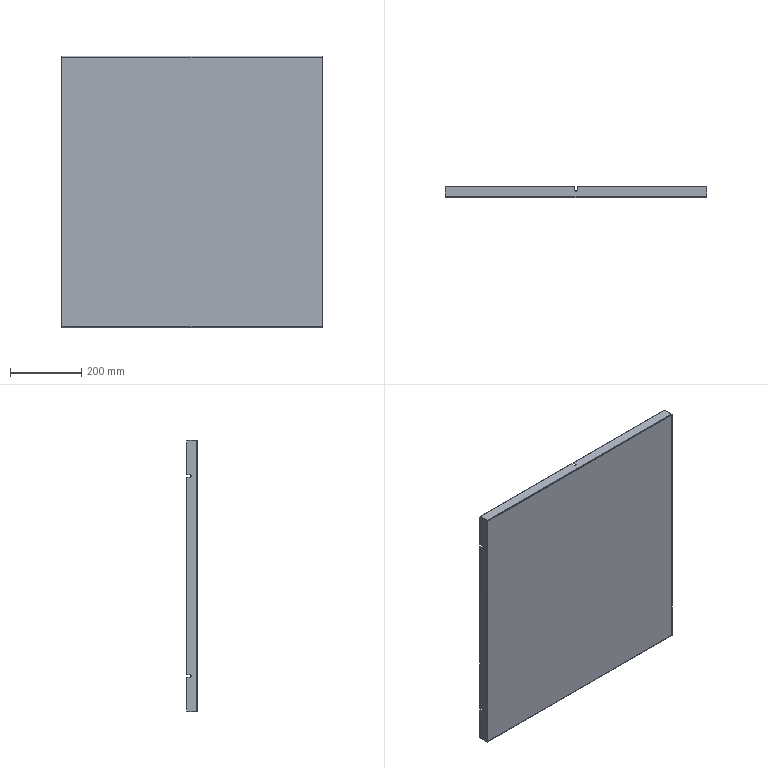Part | STEP file | JBJ-P-1011-08 | 1 solid | 62 faces | box 735 x 30 x 762 mm | volume 771967 mm3 | plane 40 | cylinder 14 | spline 8 | commonest cylinder face diameters 6.5 x6 2 x4 4.4 x4